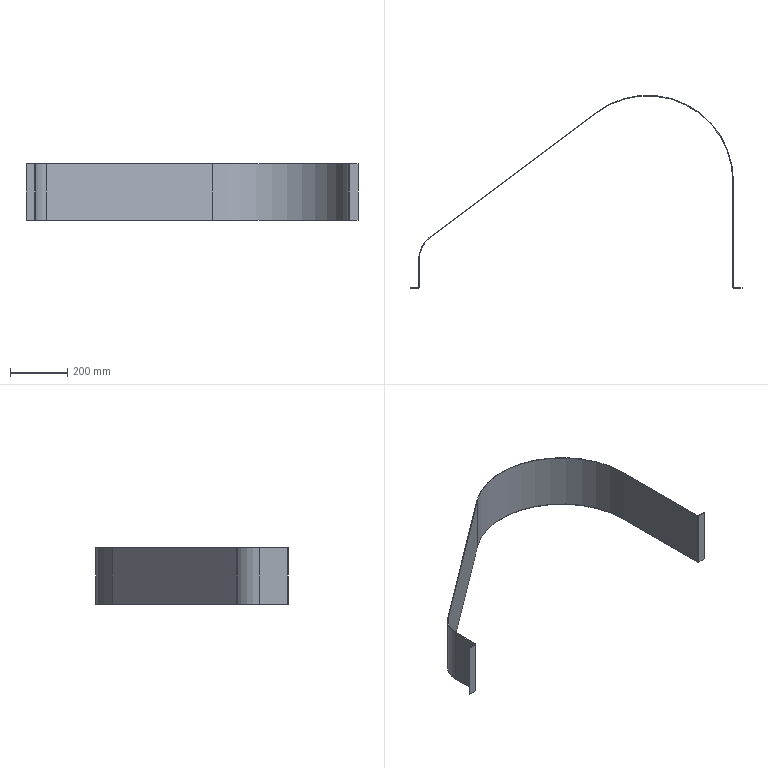Part | SolidWorks | features ICE 5, SheetMetal 3, SolidToSheetMetal 3, DeleteBody 1, Extrusion 1, FlatPattern 1, Shell 1, Split 1 | 1 solid | 38 faces | box 1160 x 675 x 198 mm | volume 796815 mm3 | plane 30 | cylinder 8 | commonest cylinder face diameters 2 x2 6 x2 196 x1 200 x1 596 x1 600 x1
STEP:
#1=CARTESIAN_POINT('',(-1098.,3.,0.));
#2=VERTEX_POINT('',#1);
#3=CARTESIAN_POINT('',(-1100.,3.,0.));
#4=VERTEX_POINT('',#3);
#5=CARTESIAN_POINT('',(-1100.,3.,0.));
#6=DIRECTION('',(-1.,0.,0.));
#7=VECTOR('',#6,1000.);
#8=LINE('',#5,#7);
#9=EDGE_CURVE('',#2,#4,#8,.T.);
#10=ORIENTED_EDGE('',*,*,#9,.F.);
#11=CARTESIAN_POINT('',(-1098.,100.,0.));
#12=VERTEX_POINT('',#11);
#13=CARTESIAN_POINT('',(-1098.,100.,0.));
#14=DIRECTION('',(0.,-1.,0.));
#15=VECTOR('',#14,1000.);
#16=LINE('',#13,#15);
#17=EDGE_CURVE('',#12,#2,#16,.T.);
#18=ORIENTED_EDGE('',*,*,#17,.F.);
#19=CARTESIAN_POINT('',(-1100.,100.,0.));
#20=VERTEX_POINT('',#19);
#21=CARTESIAN_POINT('',(-1100.,100.,0.));
#22=DIRECTION('',(-1.,0.,0.));
#23=VECTOR('',#22,1000.);
#24=LINE('',#21,#23);
#25=EDGE_CURVE('',#12,#20,#24,.T.);
#26=ORIENTED_EDGE('',*,*,#25,.T.);
#27=CARTESIAN_POINT('',(-1100.,100.,0.));
#28=DIRECTION('',(0.,-1.,0.));
#29=VECTOR('',#28,1000.);
#30=LINE('',#27,#29);
#31=EDGE_CURVE('',#20,#4,#30,.T.);
#32=ORIENTED_EDGE('',*,*,#31,.T.);
#33=EDGE_LOOP('',(#10,#18,#26,#32));
#34=FACE_OUTER_BOUND('',#33,.T.);
#35=CARTESIAN_POINT('',(-1100.,100.,0.));
#36=DIRECTION('',(0.,0.,-1.));
#37=DIRECTION('',(0.,-1.,0.));
#38=AXIS2_PLACEMENT_3D('',#35,#36,#37);
#39=PLANE('',#38);
#40=ADVANCED_FACE('',(#34),#39,.F.);
#41=ORIENTED_EDGE('',*,*,#25,.F.);
#42=CARTESIAN_POINT('',(-1058.8,178.4,0.));
#43=VERTEX_POINT('',#42);
#44=CARTESIAN_POINT('',(-1000.,100.,0.));
#45=DIRECTION('',(0.,0.,1.));
#46=DIRECTION('',(1.,0.,0.));
#47=AXIS2_PLACEMENT_3D('',#44,#45,#46);
#48=CIRCLE('',#47,98.);
#49=EDGE_CURVE('',#43,#12,#48,.T.);
#50=ORIENTED_EDGE('',*,*,#49,.F.);
#51=CARTESIAN_POINT('',(-1060.,180.,0.));
#52=VERTEX_POINT('',#51);
#53=CARTESIAN_POINT('',(-1060.,180.,0.));
#54=DIRECTION('',(-0.6,0.8,0.));
#55=VECTOR('',#54,1000.);
#56=LINE('',#53,#55);
#57=EDGE_CURVE('',#43,#52,#56,.T.);
#58=ORIENTED_EDGE('',*,*,#57,.T.);
#59=CARTESIAN_POINT('',(-1000.,100.,0.));
#60=DIRECTION('',(0.,0.,1.));
#61=DIRECTION('',(1.,0.,0.));
#62=AXIS2_PLACEMENT_3D('',#59,#60,#61);
#63=CIRCLE('',#62,100.);
#64=EDGE_CURVE('',#52,#20,#63,.T.);
#65=ORIENTED_EDGE('',*,*,#64,.T.);
#66=EDGE_LOOP('',(#41,#50,#58,#65));
#67=FACE_OUTER_BOUND('',#66,.T.);
#68=CARTESIAN_POINT('',(-1000.,100.,0.));
#69=DIRECTION('',(0.,0.,-1.));
#70=DIRECTION('',(-1.,0.,0.));
#71=AXIS2_PLACEMENT_3D('',#68,#69,#70);
#72=PLANE('',#71);
#73=ADVANCED_FACE('',(#67),#72,.F.);
#74=ORIENTED_EDGE('',*,*,#57,.F.);
#75=CARTESIAN_POINT('',(-478.8,613.4,0.));
#76=VERTEX_POINT('',#75);
#77=CARTESIAN_POINT('',(-1058.8,178.4,0.));
#78=DIRECTION('',(-0.8,-0.6,0.));
#79=VECTOR('',#78,1000.);
#80=LINE('',#77,#79);
#81=EDGE_CURVE('',#76,#43,#80,.T.);
#82=ORIENTED_EDGE('',*,*,#81,.F.);
#83=CARTESIAN_POINT('',(-480.,615.,0.));
#84=VERTEX_POINT('',#83);
#85=CARTESIAN_POINT('',(-480.,615.,0.));
#86=DIRECTION('',(-0.6,0.8,0.));
#87=VECTOR('',#86,1000.);
#88=LINE('',#85,#87);
#89=EDGE_CURVE('',#76,#84,#88,.T.);
#90=ORIENTED_EDGE('',*,*,#89,.T.);
#91=CARTESIAN_POINT('',(-1060.,180.,0.));
#92=DIRECTION('',(-0.8,-0.6,0.));
#93=VECTOR('',#92,1000.);
#94=LINE('',#91,#93);
#95=EDGE_CURVE('',#84,#52,#94,.T.);
#96=ORIENTED_EDGE('',*,*,#95,.T.);
#97=EDGE_LOOP('',(#74,#82,#90,#96));
#98=FACE_OUTER_BOUND('',#97,.T.);
#99=CARTESIAN_POINT('',(-1060.,180.,0.));
#100=DIRECTION('',(0.,0.,-1.));
#101=DIRECTION('',(-0.8,-0.6,0.));
#102=AXIS2_PLACEMENT_3D('',#99,#100,#101);
#103=PLANE('',#102);
#104=ADVANCED_FACE('',(#98),#103,.F.);
#105=ORIENTED_EDGE('',*,*,#89,.F.);
#106=CARTESIAN_POINT('',(-2.,375.,0.));
#107=VERTEX_POINT('',#106);
#108=CARTESIAN_POINT('',(-300.,375.,0.));
#109=DIRECTION('',(0.,0.,1.));
#110=DIRECTION('',(1.,0.,0.));
#111=AXIS2_PLACEMENT_3D('',#108,#109,#110);
#112=CIRCLE('',#111,298.);
#113=EDGE_CURVE('',#107,#76,#112,.T.);
#114=ORIENTED_EDGE('',*,*,#113,.F.);
#115=CARTESIAN_POINT('',(0.,375.,0.));
#116=VERTEX_POINT('',#115);
#117=CARTESIAN_POINT('',(0.,375.,0.));
#118=DIRECTION('',(1.,0.,0.));
#119=VECTOR('',#118,1000.);
#120=LINE('',#117,#119);
#121=EDGE_CURVE('',#107,#116,#120,.T.);
#122=ORIENTED_EDGE('',*,*,#121,.T.);
#123=CARTESIAN_POINT('',(-300.,375.,0.));
#124=DIRECTION('',(0.,0.,1.));
#125=DIRECTION('',(1.,0.,0.));
#126=AXIS2_PLACEMENT_3D('',#123,#124,#125);
#127=CIRCLE('',#126,300.);
#128=EDGE_CURVE('',#116,#84,#127,.T.);
#129=ORIENTED_EDGE('',*,*,#128,.T.);
#130=EDGE_LOOP('',(#105,#114,#122,#129));
#131=FACE_OUTER_BOUND('',#130,.T.);
#132=CARTESIAN_POINT('',(-300.,375.,0.));
#133=DIRECTION('',(0.,0.,-1.));
#134=DIRECTION('',(-1.,0.,0.));
#135=AXIS2_PLACEMENT_3D('',#132,#133,#134);
#136=PLANE('',#135);
#137=ADVANCED_FACE('',(#131),#136,.F.);
#138=ORIENTED_EDGE('',*,*,#121,.F.);
#139=CARTESIAN_POINT('',(-2.,3.,0.));
#140=VERTEX_POINT('',#139);
#141=CARTESIAN_POINT('',(-2.,0.,0.));
#142=DIRECTION('',(0.,1.,0.));
#143=VECTOR('',#142,1000.);
#144=LINE('',#141,#143);
#145=EDGE_CURVE('',#140,#107,#144,.T.);
#146=ORIENTED_EDGE('',*,*,#145,.F.);
#147=CARTESIAN_POINT('',(0.,3.,0.));
#148=VERTEX_POINT('',#147);
#149=CARTESIAN_POINT('',(0.,3.,0.));
#150=DIRECTION('',(1.,0.,0.));
#151=VECTOR('',#150,1000.);
#152=LINE('',#149,#151);
#153=EDGE_CURVE('',#140,#148,#152,.T.);
#154=ORIENTED_EDGE('',*,*,#153,.T.);
#155=CARTESIAN_POINT('',(0.,0.,0.));
#156=DIRECTION('',(0.,1.,0.));
#157=VECTOR('',#156,1000.);
#158=LINE('',#155,#157);
#159=EDGE_CURVE('',#148,#116,#158,.T.);
#160=ORIENTED_EDGE('',*,*,#159,.T.);
#161=EDGE_LOOP('',(#138,#146,#154,#160));
#162=FACE_OUTER_BOUND('',#161,.T.);
#163=CARTESIAN_POINT('',(0.,0.,0.));
#164=DIRECTION('',(0.,0.,-1.));
#165=DIRECTION('',(0.,1.,0.));
#166=AXIS2_PLACEMENT_3D('',#163,#164,#165);
#167=PLANE('',#166);
#168=ADVANCED_FACE('',(#162),#167,.F.);
#169=ORIENTED_EDGE('',*,*,#153,.F.);
#170=CARTESIAN_POINT('',(1.,0.,0.));
#171=VERTEX_POINT('',#170);
#172=CARTESIAN_POINT('',(1.,3.,0.));
#173=DIRECTION('',(0.,0.,1.));
#174=DIRECTION('',(1.,0.,0.));
#175=AXIS2_PLACEMENT_3D('',#172,#173,#174);
#176=CIRCLE('',#175,3.);
#177=EDGE_CURVE('',#140,#171,#176,.T.);
#178=ORIENTED_EDGE('',*,*,#177,.T.);
#179=CARTESIAN_POINT('',(1.,2.,0.));
#180=VERTEX_POINT('',#179);
#181=CARTESIAN_POINT('',(1.,2.,0.));
#182=DIRECTION('',(0.,1.,0.));
#183=VECTOR('',#182,1000.);
#184=LINE('',#181,#183);
#185=EDGE_CURVE('',#171,#180,#184,.T.);
#186=ORIENTED_EDGE('',*,*,#185,.T.);
#187=CARTESIAN_POINT('',(1.,3.,0.));
#188=DIRECTION('',(0.,0.,1.));
#189=DIRECTION('',(-1.,0.,0.));
#190=AXIS2_PLACEMENT_3D('',#187,#188,#189);
#191=CIRCLE('',#190,1.);
#192=EDGE_CURVE('',#148,#180,#191,.T.);
#193=ORIENTED_EDGE('',*,*,#192,.F.);
#194=EDGE_LOOP('',(#169,#178,#186,#193));
#195=FACE_OUTER_BOUND('',#194,.T.);
#196=CARTESIAN_POINT('',(1.,3.,0.));
#197=DIRECTION('',(0.,0.,1.));
#198=DIRECTION('',(1.,0.,0.));
#199=AXIS2_PLACEMENT_3D('',#196,#197,#198);
#200=PLANE('',#199);
#201=ADVANCED_FACE('',(#195),#200,.T.);
#202=ORIENTED_EDGE('',*,*,#185,.F.);
#203=CARTESIAN_POINT('',(30.,0.,0.));
#204=VERTEX_POINT('',#203);
#205=CARTESIAN_POINT('',(0.,0.,0.));
#206=DIRECTION('',(-1.,0.,0.));
#207=VECTOR('',#206,1000.);
#208=LINE('',#205,#207);
#209=EDGE_CURVE('',#204,#171,#208,.T.);
#210=ORIENTED_EDGE('',*,*,#209,.F.);
#211=CARTESIAN_POINT('',(30.,2.,0.));
#212=VERTEX_POINT('',#211);
#213=CARTESIAN_POINT('',(30.,2.,0.));
#214=DIRECTION('',(0.,1.,0.));
#215=VECTOR('',#214,1000.);
#216=LINE('',#213,#215);
#217=EDGE_CURVE('',#204,#212,#216,.T.);
#218=ORIENTED_EDGE('',*,*,#217,.T.);
#219=CARTESIAN_POINT('',(30.,2.,0.));
#220=DIRECTION('',(-1.,0.,0.));
#221=VECTOR('',#220,1000.);
#222=LINE('',#219,#221);
#223=EDGE_CURVE('',#212,#180,#222,.T.);
#224=ORIENTED_EDGE('',*,*,#223,.T.);
#225=EDGE_LOOP('',(#202,#210,#218,#224));
#226=FACE_OUTER_BOUND('',#225,.T.);
#227=CARTESIAN_POINT('',(30.,2.,0.));
#228=DIRECTION('',(0.,0.,-1.));
#229=DIRECTION('',(-1.,0.,0.));
#230=AXIS2_PLACEMENT_3D('',#227,#228,#229);
#231=PLANE('',#230);
#232=ADVANCED_FACE('',(#226),#231,.F.);
#233=ORIENTED_EDGE('',*,*,#217,.F.);
#234=CARTESIAN_POINT('',(30.,0.,-198.));
#235=VERTEX_POINT('',#234);
#236=CARTESIAN_POINT('',(30.,0.,0.));
#237=DIRECTION('',(0.,0.,1.));
#238=VECTOR('',#237,1000.);
#239=LINE('',#236,#238);
#240=EDGE_CURVE('',#235,#204,#239,.T.);
#241=ORIENTED_EDGE('',*,*,#240,.F.);
#242=CARTESIAN_POINT('',(30.,2.,-198.));
#243=VERTEX_POINT('',#242);
#244=CARTESIAN_POINT('',(30.,2.,-198.));
#245=DIRECTION('',(0.,1.,0.));
#246=VECTOR('',#245,1000.);
#247=LINE('',#244,#246);
#248=EDGE_CURVE('',#235,#243,#247,.T.);
#249=ORIENTED_EDGE('',*,*,#248,.T.);
#250=CARTESIAN_POINT('',(30.,2.,-230.));
#251=DIRECTION('',(0.,0.,1.));
#252=VECTOR('',#251,1000.);
#253=LINE('',#250,#252);
#254=EDGE_CURVE('',#243,#212,#253,.T.);
#255=ORIENTED_EDGE('',*,*,#254,.T.);
#256=EDGE_LOOP('',(#233,#241,#249,#255));
#257=FACE_OUTER_BOUND('',#256,.T.);
#258=CARTESIAN_POINT('',(30.,2.,-230.));
#259=DIRECTION('',(-1.,0.,0.));
#260=DIRECTION('',(0.,0.,1.));
#261=AXIS2_PLACEMENT_3D('',#258,#259,#260);
#262=PLANE('',#261);
#263=ADVANCED_FACE('',(#257),#262,.F.);
#264=ORIENTED_EDGE('',*,*,#248,.F.);
#265=CARTESIAN_POINT('',(1.,0.,-198.));
#266=VERTEX_POINT('',#265);
#267=CARTESIAN_POINT('',(0.,0.,-198.));
#268=DIRECTION('',(1.,0.,0.));
#269=VECTOR('',#268,1000.);
#270=LINE('',#267,#269);
#271=EDGE_CURVE('',#266,#235,#270,.T.);
#272=ORIENTED_EDGE('',*,*,#271,.F.);
#273=CARTESIAN_POINT('',(1.,2.,-198.));
#274=VERTEX_POINT('',#273);
#275=CARTESIAN_POINT('',(1.,2.,-198.));
#276=DIRECTION('',(0.,1.,0.));
#277=VECTOR('',#276,1000.);
#278=LINE('',#275,#277);
#279=EDGE_CURVE('',#266,#274,#278,.T.);
#280=ORIENTED_EDGE('',*,*,#279,.T.);
#281=CARTESIAN_POINT('',(0.,2.,-198.));
#282=DIRECTION('',(1.,0.,0.));
#283=VECTOR('',#282,1000.);
#284=LINE('',#281,#283);
#285=EDGE_CURVE('',#274,#243,#284,.T.);
#286=ORIENTED_EDGE('',*,*,#285,.T.);
#287=EDGE_LOOP('',(#264,#272,#280,#286));
#288=FACE_OUTER_BOUND('',#287,.T.);
#289=CARTESIAN_POINT('',(0.,2.,-198.));
#290=DIRECTION('',(0.,0.,1.));
#291=DIRECTION('',(1.,0.,0.));
#292=AXIS2_PLACEMENT_3D('',#289,#290,#291);
#293=PLANE('',#292);
#294=ADVANCED_FACE('',(#288),#293,.F.);
#295=ORIENTED_EDGE('',*,*,#279,.F.);
#296=CARTESIAN_POINT('',(-2.,3.,-198.));
#297=VERTEX_POINT('',#296);
#298=CARTESIAN_POINT('',(1.,3.,-198.));
#299=DIRECTION('',(0.,0.,-1.));
#300=DIRECTION('',(1.,0.,0.));
#301=AXIS2_PLACEMENT_3D('',#298,#299,#300);
#302=CIRCLE('',#301,3.);
#303=EDGE_CURVE('',#266,#297,#302,.T.);
#304=ORIENTED_EDGE('',*,*,#303,.T.);
#305=CARTESIAN_POINT('',(0.,3.,-198.));
#306=VERTEX_POINT('',#305);
#307=CARTESIAN_POINT('',(0.,3.,-198.));
#308=DIRECTION('',(1.,0.,0.));
#309=VECTOR('',#308,1000.);
#310=LINE('',#307,#309);
#311=EDGE_CURVE('',#297,#306,#310,.T.);
#312=ORIENTED_EDGE('',*,*,#311,.T.);
#313=CARTESIAN_POINT('',(1.,3.,-198.));
#314=DIRECTION('',(0.,0.,-1.));
#315=DIRECTION('',(1.,0.,0.));
#316=AXIS2_PLACEMENT_3D('',#313,#314,#315);
#317=CIRCLE('',#316,1.);
#318=EDGE_CURVE('',#274,#306,#317,.T.);
#319=ORIENTED_EDGE('',*,*,#318,.F.);
#320=EDGE_LOOP('',(#295,#304,#312,#319));
#321=FACE_OUTER_BOUND('',#320,.T.);
#322=CARTESIAN_POINT('',(1.,3.,-198.));
#323=DIRECTION('',(0.,0.,-1.));
#324=DIRECTION('',(-1.,0.,0.));
#325=AXIS2_PLACEMENT_3D('',#322,#323,#324);
#326=PLANE('',#325);
#327=ADVANCED_FACE('',(#321),#326,.T.);
#328=ORIENTED_EDGE('',*,*,#311,.F.);
#329=CARTESIAN_POINT('',(-2.,375.,-198.));
#330=VERTEX_POINT('',#329);
#331=CARTESIAN_POINT('',(-2.,0.,-198.));
#332=DIRECTION('',(0.,-1.,0.));
#333=VECTOR('',#332,1000.);
#334=LINE('',#331,#333);
#335=EDGE_CURVE('',#330,#297,#334,.T.);
#336=ORIENTED_EDGE('',*,*,#335,.F.);
#337=CARTESIAN_POINT('',(0.,375.,-198.));
#338=VERTEX_POINT('',#337);
#339=CARTESIAN_POINT('',(0.,375.,-198.));
#340=DIRECTION('',(1.,0.,0.));
#341=VECTOR('',#340,1000.);
#342=LINE('',#339,#341);
#343=EDGE_CURVE('',#330,#338,#342,.T.);
#344=ORIENTED_EDGE('',*,*,#343,.T.);
#345=CARTESIAN_POINT('',(0.,0.,-198.));
#346=DIRECTION('',(0.,-1.,0.));
#347=VECTOR('',#346,1000.);
#348=LINE('',#345,#347);
#349=EDGE_CURVE('',#338,#306,#348,.T.);
#350=ORIENTED_EDGE('',*,*,#349,.T.);
#351=EDGE_LOOP('',(#328,#336,#344,#350));
#352=FACE_OUTER_BOUND('',#351,.T.);
#353=CARTESIAN_POINT('',(0.,0.,-198.));
#354=DIRECTION('',(0.,0.,1.));
#355=DIRECTION('',(0.,-1.,0.));
#356=AXIS2_PLACEMENT_3D('',#353,#354,#355);
#357=PLANE('',#356);
#358=ADVANCED_FACE('',(#352),#357,.F.);
#359=ORIENTED_EDGE('',*,*,#343,.F.);
#360=CARTESIAN_POINT('',(-478.8,613.4,-198.));
#361=VERTEX_POINT('',#360);
#362=CARTESIAN_POINT('',(-300.,375.,-198.));
#363=DIRECTION('',(0.,0.,-1.));
#364=DIRECTION('',(1.,0.,0.));
#365=AXIS2_PLACEMENT_3D('',#362,#363,#364);
#366=CIRCLE('',#365,298.);
#367=EDGE_CURVE('',#361,#330,#366,.T.);
#368=ORIENTED_EDGE('',*,*,#367,.F.);
#369=CARTESIAN_POINT('',(-480.,615.,-198.));
#370=VERTEX_POINT('',#369);
#371=CARTESIAN_POINT('',(-480.,615.,-198.));
#372=DIRECTION('',(-0.6,0.8,0.));
#373=VECTOR('',#372,1000.);
#374=LINE('',#371,#373);
#375=EDGE_CURVE('',#361,#370,#374,.T.);
#376=ORIENTED_EDGE('',*,*,#375,.T.);
#377=CARTESIAN_POINT('',(-300.,375.,-198.));
#378=DIRECTION('',(0.,0.,-1.));
#379=DIRECTION('',(1.,0.,0.));
#380=AXIS2_PLACEMENT_3D('',#377,#378,#379);
#381=CIRCLE('',#380,300.);
#382=EDGE_CURVE('',#370,#338,#381,.T.);
#383=ORIENTED_EDGE('',*,*,#382,.T.);
#384=EDGE_LOOP('',(#359,#368,#376,#383));
#385=FACE_OUTER_BOUND('',#384,.T.);
#386=CARTESIAN_POINT('',(-300.,375.,-198.));
#387=DIRECTION('',(0.,0.,-1.));
#388=DIRECTION('',(-1.,0.,0.));
#389=AXIS2_PLACEMENT_3D('',#386,#387,#388);
#390=PLANE('',#389);
#391=ADVANCED_FACE('',(#385),#390,.T.);
#392=ORIENTED_EDGE('',*,*,#375,.F.);
#393=CARTESIAN_POINT('',(-1058.8,178.4,-198.));
#394=VERTEX_POINT('',#393);
#395=CARTESIAN_POINT('',(-1058.8,178.4,-198.));
#396=DIRECTION('',(0.8,0.6,0.));
#397=VECTOR('',#396,1000.);
#398=LINE('',#395,#397);
#399=EDGE_CURVE('',#394,#361,#398,.T.);
#400=ORIENTED_EDGE('',*,*,#399,.F.);
#401=CARTESIAN_POINT('',(-1060.,180.,-198.));
#402=VERTEX_POINT('',#401);
#403=CARTESIAN_POINT('',(-1060.,180.,-198.));
#404=DIRECTION('',(-0.6,0.8,0.));
#405=VECTOR('',#404,1000.);
#406=LINE('',#403,#405);
#407=EDGE_CURVE('',#394,#402,#406,.T.);
#408=ORIENTED_EDGE('',*,*,#407,.T.);
#409=CARTESIAN_POINT('',(-1060.,180.,-198.));
#410=DIRECTION('',(0.8,0.6,0.));
#411=VECTOR('',#410,1000.);
#412=LINE('',#409,#411);
#413=EDGE_CURVE('',#402,#370,#412,.T.);
#414=ORIENTED_EDGE('',*,*,#413,.T.);
#415=EDGE_LOOP('',(#392,#400,#408,#414));
#416=FACE_OUTER_BOUND('',#415,.T.);
#417=CARTESIAN_POINT('',(-1060.,180.,-198.));
#418=DIRECTION('',(0.,0.,1.));
#419=DIRECTION('',(0.8,0.6,0.));
#420=AXIS2_PLACEMENT_3D('',#417,#418,#419);
#421=PLANE('',#420);
#422=ADVANCED_FACE('',(#416),#421,.F.);
#423=ORIENTED_EDGE('',*,*,#407,.F.);
#424=CARTESIAN_POINT('',(-1098.,100.,-198.));
#425=VERTEX_POINT('',#424);
#426=CARTESIAN_POINT('',(-1000.,100.,-198.));
#427=DIRECTION('',(0.,0.,-1.));
#428=DIRECTION('',(1.,0.,0.));
#429=AXIS2_PLACEMENT_3D('',#426,#427,#428);
#430=CIRCLE('',#429,98.);
#431=EDGE_CURVE('',#425,#394,#430,.T.);
#432=ORIENTED_EDGE('',*,*,#431,.F.);
#433=CARTESIAN_POINT('',(-1100.,100.,-198.));
#434=VERTEX_POINT('',#433);
#435=CARTESIAN_POINT('',(-1100.,100.,-198.));
#436=DIRECTION('',(-1.,0.,0.));
#437=VECTOR('',#436,1000.);
#438=LINE('',#435,#437);
#439=EDGE_CURVE('',#425,#434,#438,.T.);
#440=ORIENTED_EDGE('',*,*,#439,.T.);
#441=CARTESIAN_POINT('',(-1000.,100.,-198.));
#442=DIRECTION('',(0.,0.,-1.));
#443=DIRECTION('',(1.,0.,0.));
#444=AXIS2_PLACEMENT_3D('',#441,#442,#443);
#445=CIRCLE('',#444,100.);
#446=EDGE_CURVE('',#434,#402,#445,.T.);
#447=ORIENTED_EDGE('',*,*,#446,.T.);
#448=EDGE_LOOP('',(#423,#432,#440,#447));
#449=FACE_OUTER_BOUND('',#448,.T.);
#450=CARTESIAN_POINT('',(-1000.,100.,-198.));
#451=DIRECTION('',(0.,0.,-1.));
#452=DIRECTION('',(-1.,0.,0.));
#453=AXIS2_PLACEMENT_3D('',#450,#451,#452);
#454=PLANE('',#453);
#455=ADVANCED_FACE('',(#449),#454,.T.);
#456=ORIENTED_EDGE('',*,*,#439,.F.);
#457=CARTESIAN_POINT('',(-1098.,3.,-198.));
#458=VERTEX_POINT('',#457);
#459=CARTESIAN_POINT('',(-1098.,100.,-198.));
#460=DIRECTION('',(0.,1.,0.));
#461=VECTOR('',#460,1000.);
#462=LINE('',#459,#461);
#463=EDGE_CURVE('',#458,#425,#462,.T.);
#464=ORIENTED_EDGE('',*,*,#463,.F.);
#465=CARTESIAN_POINT('',(-1100.,3.,-198.));
#466=VERTEX_POINT('',#465);
#467=CARTESIAN_POINT('',(-1100.,3.,-198.));
#468=DIRECTION('',(-1.,0.,0.));
#469=VECTOR('',#468,1000.);
#470=LINE('',#467,#469);
#471=EDGE_CURVE('',#458,#466,#470,.T.);
#472=ORIENTED_EDGE('',*,*,#471,.T.);
#473=CARTESIAN_POINT('',(-1100.,100.,-198.));
#474=DIRECTION('',(0.,1.,0.));
#475=VECTOR('',#474,1000.);
#476=LINE('',#473,#475);
#477=EDGE_CURVE('',#466,#434,#476,.T.);
#478=ORIENTED_EDGE('',*,*,#477,.T.);
#479=EDGE_LOOP('',(#456,#464,#472,#478));
#480=FACE_OUTER_BOUND('',#479,.T.);
#481=CARTESIAN_POINT('',(-1100.,100.,-198.));
#482=DIRECTION('',(0.,0.,1.));
#483=DIRECTION('',(0.,1.,0.));
#484=AXIS2_PLACEMENT_3D('',#481,#482,#483);
#485=PLANE('',#484);
#486=ADVANCED_FACE('',(#480),#485,.F.);
#487=ORIENTED_EDGE('',*,*,#471,.F.);
#488=CARTESIAN_POINT('',(-1101.,0.,-198.));
#489=VERTEX_POINT('',#488);
#490=CARTESIAN_POINT('',(-1101.,3.,-198.));
#491=DIRECTION('',(0.,0.,-1.));
#492=DIRECTION('',(-1.,0.,0.));
#493=AXIS2_PLACEMENT_3D('',#490,#491,#492);
#494=CIRCLE('',#493,3.);
#495=EDGE_CURVE('',#458,#489,#494,.T.);
#496=ORIENTED_EDGE('',*,*,#495,.T.);
#497=CARTESIAN_POINT('',(-1101.,2.,-198.));
#498=VERTEX_POINT('',#497);
#499=CARTESIAN_POINT('',(-1101.,2.,-198.));
#500=DIRECTION('',(0.,1.,0.));
#501=VECTOR('',#500,1000.);
#502=LINE('',#499,#501);
#503=EDGE_CURVE('',#489,#498,#502,.T.);
#504=ORIENTED_EDGE('',*,*,#503,.T.);
#505=CARTESIAN_POINT('',(-1101.,3.,-198.));
#506=DIRECTION('',(0.,0.,-1.));
#507=DIRECTION('',(1.,0.,0.));
#508=AXIS2_PLACEMENT_3D('',#505,#506,#507);
#509=CIRCLE('',#508,1.);
#510=EDGE_CURVE('',#466,#498,#509,.T.);
#511=ORIENTED_EDGE('',*,*,#510,.F.);
#512=EDGE_LOOP('',(#487,#496,#504,#511));
#513=FACE_OUTER_BOUND('',#512,.T.);
#514=CARTESIAN_POINT('',(-1101.,3.,-198.));
#515=DIRECTION('',(0.,0.,-1.));
#516=DIRECTION('',(-1.,0.,0.));
#517=AXIS2_PLACEMENT_3D('',#514,#515,#516);
#518=PLANE('',#517);
#519=ADVANCED_FACE('',(#513),#518,.T.);
#520=ORIENTED_EDGE('',*,*,#503,.F.);
#521=CARTESIAN_POINT('',(-1130.,0.,-198.));
#522=VERTEX_POINT('',#521);
#523=CARTESIAN_POINT('',(0.,0.,-198.));
#524=DIRECTION('',(1.,0.,0.));
#525=VECTOR('',#524,1000.);
#526=LINE('',#523,#525);
#527=EDGE_CURVE('',#522,#489,#526,.T.);
#528=ORIENTED_EDGE('',*,*,#527,.F.);
#529=CARTESIAN_POINT('',(-1130.,2.,-198.));
#530=VERTEX_POINT('',#529);
#531=CARTESIAN_POINT('',(-1130.,2.,-198.));
#532=DIRECTION('',(0.,1.,0.));
#533=VECTOR('',#532,1000.);
#534=LINE('',#531,#533);
#535=EDGE_CURVE('',#522,#530,#534,.T.);
#536=ORIENTED_EDGE('',*,*,#535,.T.);
#537=CARTESIAN_POINT('',(0.,2.,-198.));
#538=DIRECTION('',(1.,0.,0.));
#539=VECTOR('',#538,1000.);
#540=LINE('',#537,#539);
#541=EDGE_CURVE('',#530,#498,#540,.T.);
#542=ORIENTED_EDGE('',*,*,#541,.T.);
#543=EDGE_LOOP('',(#520,#528,#536,#542));
#544=FACE_OUTER_BOUND('',#543,.T.);
#545=CARTESIAN_POINT('',(0.,2.,-198.));
#546=DIRECTION('',(0.,0.,1.));
#547=DIRECTION('',(1.,0.,0.));
#548=AXIS2_PLACEMENT_3D('',#545,#546,#547);
#549=PLANE('',#548);
#550=ADVANCED_FACE('',(#544),#549,.F.);
#551=ORIENTED_EDGE('',*,*,#535,.F.);
#552=CARTESIAN_POINT('',(-1130.,0.,0.));
#553=VERTEX_POINT('',#552);
#554=CARTESIAN_POINT('',(-1130.,0.,0.));
#555=DIRECTION('',(0.,0.,-1.));
#556=VECTOR('',#555,1000.);
#557=LINE('',#554,#556);
#558=EDGE_CURVE('',#553,#522,#557,.T.);
#559=ORIENTED_EDGE('',*,*,#558,.F.);
#560=CARTESIAN_POINT('',(-1130.,2.,0.));
#561=VERTEX_POINT('',#560);
#562=CARTESIAN_POINT('',(-1130.,2.,0.));
#563=DIRECTION('',(0.,1.,0.));
#564=VECTOR('',#563,1000.);
#565=LINE('',#562,#564);
#566=EDGE_CURVE('',#553,#561,#565,.T.);
#567=ORIENTED_EDGE('',*,*,#566,.T.);
#568=CARTESIAN_POINT('',(-1130.,2.,0.));
#569=DIRECTION('',(0.,0.,-1.));
#570=VECTOR('',#569,1000.);
#571=LINE('',#568,#570);
#572=EDGE_CURVE('',#561,#530,#571,.T.);
#573=ORIENTED_EDGE('',*,*,#572,.T.);
#574=EDGE_LOOP('',(#551,#559,#567,#573));
#575=FACE_OUTER_BOUND('',#574,.T.);
#576=CARTESIAN_POINT('',(-1130.,2.,0.));
#577=DIRECTION('',(1.,0.,0.));
#578=DIRECTION('',(0.,0.,-1.));
#579=AXIS2_PLACEMENT_3D('',#576,#577,#578);
#580=PLANE('',#579);
#581=ADVANCED_FACE('',(#575),#580,.F.);
#582=ORIENTED_EDGE('',*,*,#566,.F.);
#583=CARTESIAN_POINT('',(-1101.,0.,0.));
#584=VERTEX_POINT('',#583);
#585=CARTESIAN_POINT('',(0.,0.,0.));
#586=DIRECTION('',(-1.,0.,0.));
#587=VECTOR('',#586,1000.);
#588=LINE('',#585,#587);
#589=EDGE_CURVE('',#584,#553,#588,.T.);
#590=ORIENTED_EDGE('',*,*,#589,.F.);
#591=CARTESIAN_POINT('',(-1101.,2.,0.));
#592=VERTEX_POINT('',#591);
#593=CARTESIAN_POINT('',(-1101.,2.,0.));
#594=DIRECTION('',(0.,1.,0.));
#595=VECTOR('',#594,1000.);
#596=LINE('',#593,#595);
#597=EDGE_CURVE('',#584,#592,#596,.T.);
#598=ORIENTED_EDGE('',*,*,#597,.T.);
#599=CARTESIAN_POINT('',(-1100.,2.,0.));
#600=DIRECTION('',(-1.,0.,0.));
#601=VECTOR('',#600,1000.);
#602=LINE('',#599,#601);
#603=EDGE_CURVE('',#592,#561,#602,.T.);
#604=ORIENTED_EDGE('',*,*,#603,.T.);
#605=EDGE_LOOP('',(#582,#590,#598,#604));
#606=FACE_OUTER_BOUND('',#605,.T.);
#607=CARTESIAN_POINT('',(-1100.,2.,0.));
#608=DIRECTION('',(0.,0.,-1.));
#609=DIRECTION('',(-1.,0.,0.));
#610=AXIS2_PLACEMENT_3D('',#607,#608,#609);
#611=PLANE('',#610);
#612=ADVANCED_FACE('',(#606),#611,.F.);
#613=CARTESIAN_POINT('',(-1101.,3.,0.));
#614=DIRECTION('',(0.,0.,1.));
#615=DIRECTION('',(-1.,0.,0.));
#616=AXIS2_PLACEMENT_3D('',#613,#614,#615);
#617=CIRCLE('',#616,3.);
#618=EDGE_CURVE('',#584,#2,#617,.T.);
#619=ORIENTED_EDGE('',*,*,#618,.T.);
#620=ORIENTED_EDGE('',*,*,#9,.T.);
#621=CARTESIAN_POINT('',(-1101.,3.,0.));
#622=DIRECTION('',(0.,0.,1.));
#623=DIRECTION('',(-1.,0.,0.));
#624=AXIS2_PLACEMENT_3D('',#621,#622,#623);
#625=CIRCLE('',#624,1.);
#626=EDGE_CURVE('',#592,#4,#625,.T.);
#627=ORIENTED_EDGE('',*,*,#626,.F.);
#628=ORIENTED_EDGE('',*,*,#597,.F.);
#629=EDGE_LOOP('',(#619,#620,#627,#628));
#630=FACE_OUTER_BOUND('',#629,.T.);
#631=CARTESIAN_POINT('',(-1101.,3.,0.));
#632=DIRECTION('',(0.,0.,1.));
#633=DIRECTION('',(1.,0.,0.));
#634=AXIS2_PLACEMENT_3D('',#631,#632,#633);
#635=PLANE('',#634);
#636=ADVANCED_FACE('',(#630),#635,.T.);
#637=ORIENTED_EDGE('',*,*,#603,.F.);
#638=CARTESIAN_POINT('',(-1101.,2.,-198.));
#639=DIRECTION('',(0.,0.,-1.));
#640=VECTOR('',#639,1000.);
#641=LINE('',#638,#640);
#642=EDGE_CURVE('',#592,#498,#641,.T.);
#643=ORIENTED_EDGE('',*,*,#642,.T.);
#644=ORIENTED_EDGE('',*,*,#541,.F.);
#645=ORIENTED_EDGE('',*,*,#572,.F.);
#646=EDGE_LOOP('',(#637,#643,#644,#645));
#647=FACE_OUTER_BOUND('',#646,.T.);
#648=CARTESIAN_POINT('',(0.,2.,0.));
#649=DIRECTION('',(0.,1.,0.));
#650=DIRECTION('',(0.,0.,1.));
#651=AXIS2_PLACEMENT_3D('',#648,#649,#650);
#652=PLANE('',#651);
#653=ADVANCED_FACE('',(#647),#652,.T.);
#654=ORIENTED_EDGE('',*,*,#446,.F.);
#655=CARTESIAN_POINT('',(-1100.,100.,-200.));
#656=DIRECTION('',(0.,0.,1.));
#657=VECTOR('',#656,1000.);
#658=LINE('',#655,#657);
#659=EDGE_CURVE('',#434,#20,#658,.T.);
#660=ORIENTED_EDGE('',*,*,#659,.T.);
#661=ORIENTED_EDGE('',*,*,#64,.F.);
#662=CARTESIAN_POINT('',(-1060.,180.,-200.));
#663=DIRECTION('',(0.,0.,1.));
#664=VECTOR('',#663,1000.);
#665=LINE('',#662,#664);
#666=EDGE_CURVE('',#402,#52,#665,.T.);
#667=ORIENTED_EDGE('',*,*,#666,.F.);
#668=EDGE_LOOP('',(#654,#660,#661,#667));
#669=FACE_OUTER_BOUND('',#668,.T.);
#670=CARTESIAN_POINT('',(-1000.,100.,-200.));
#671=DIRECTION('',(0.,0.,1.));
#672=DIRECTION('',(1.,0.,0.));
#673=AXIS2_PLACEMENT_3D('',#670,#671,#672);
#674=CYLINDRICAL_SURFACE('',#673,100.);
#675=ADVANCED_FACE('',(#669),#674,.T.);
#676=ORIENTED_EDGE('',*,*,#477,.F.);
#677=CARTESIAN_POINT('',(-1100.,3.,0.));
#678=DIRECTION('',(0.,0.,1.));
#679=VECTOR('',#678,1000.);
#680=LINE('',#677,#679);
#681=EDGE_CURVE('',#466,#4,#680,.T.);
#682=ORIENTED_EDGE('',*,*,#681,.T.);
#683=ORIENTED_EDGE('',*,*,#31,.F.);
#684=ORIENTED_EDGE('',*,*,#659,.F.);
#685=EDGE_LOOP('',(#676,#682,#683,#684));
#686=FACE_OUTER_BOUND('',#685,.T.);
#687=CARTESIAN_POINT('',(-1100.,100.,-200.));
#688=DIRECTION('',(-1.,0.,0.));
#689=DIRECTION('',(0.,0.,1.));
#690=AXIS2_PLACEMENT_3D('',#687,#688,#689);
#691=PLANE('',#690);
#692=ADVANCED_FACE('',(#686),#691,.T.);
#693=ORIENTED_EDGE('',*,*,#382,.F.);
#694=CARTESIAN_POINT('',(-480.,615.,-200.));
#695=DIRECTION('',(0.,0.,1.));
#696=VECTOR('',#695,1000.);
#697=LINE('',#694,#696);
#698=EDGE_CURVE('',#370,#84,#697,.T.);
#699=ORIENTED_EDGE('',*,*,#698,.T.);
#700=ORIENTED_EDGE('',*,*,#128,.F.);
#701=CARTESIAN_POINT('',(0.,375.,-200.));
#702=DIRECTION('',(0.,0.,1.));
#703=VECTOR('',#702,1000.);
#704=LINE('',#701,#703);
#705=EDGE_CURVE('',#338,#116,#704,.T.);
#706=ORIENTED_EDGE('',*,*,#705,.F.);
#707=EDGE_LOOP('',(#693,#699,#700,#706));
#708=FACE_OUTER_BOUND('',#707,.T.);
#709=CARTESIAN_POINT('',(-300.,375.,-200.));
#710=DIRECTION('',(0.,0.,1.));
#711=DIRECTION('',(1.,0.,0.));
#712=AXIS2_PLACEMENT_3D('',#709,#710,#711);
#713=CYLINDRICAL_SURFACE('',#712,300.);
#714=ADVANCED_FACE('',(#708),#713,.T.);
#715=ORIENTED_EDGE('',*,*,#413,.F.);
#716=ORIENTED_EDGE('',*,*,#666,.T.);
#717=ORIENTED_EDGE('',*,*,#95,.F.);
#718=ORIENTED_EDGE('',*,*,#698,.F.);
#719=EDGE_LOOP('',(#715,#716,#717,#718));
#720=FACE_OUTER_BOUND('',#719,.T.);
#721=CARTESIAN_POINT('',(-1060.,180.,-200.));
#722=DIRECTION('',(-0.6,0.8,0.));
#723=DIRECTION('',(-0.8,-0.6,0.));
#724=AXIS2_PLACEMENT_3D('',#721,#722,#723);
#725=PLANE('',#724);
#726=ADVANCED_FACE('',(#720),#725,.T.);
#727=ORIENTED_EDGE('',*,*,#285,.F.);
#728=CARTESIAN_POINT('',(1.,2.,0.));
#729=DIRECTION('',(0.,0.,1.));
#730=VECTOR('',#729,1000.);
#731=LINE('',#728,#730);
#732=EDGE_CURVE('',#274,#180,#731,.T.);
#733=ORIENTED_EDGE('',*,*,#732,.T.);
#734=ORIENTED_EDGE('',*,*,#223,.F.);
#735=ORIENTED_EDGE('',*,*,#254,.F.);
#736=EDGE_LOOP('',(#727,#733,#734,#735));
#737=FACE_OUTER_BOUND('',#736,.T.);
#738=CARTESIAN_POINT('',(0.,2.,0.));
#739=DIRECTION('',(0.,1.,0.));
#740=DIRECTION('',(0.,0.,1.));
#741=AXIS2_PLACEMENT_3D('',#738,#739,#740);
#742=PLANE('',#741);
#743=ADVANCED_FACE('',(#737),#742,.T.);
#744=ORIENTED_EDGE('',*,*,#159,.F.);
#745=CARTESIAN_POINT('',(0.,3.,-198.));
#746=DIRECTION('',(0.,0.,-1.));
#747=VECTOR('',#746,1000.);
#748=LINE('',#745,#747);
#749=EDGE_CURVE('',#148,#306,#748,.T.);
#750=ORIENTED_EDGE('',*,*,#749,.T.);
#751=ORIENTED_EDGE('',*,*,#349,.F.);
#752=ORIENTED_EDGE('',*,*,#705,.T.);
#753=EDGE_LOOP('',(#744,#750,#751,#752));
#754=FACE_OUTER_BOUND('',#753,.T.);
#755=CARTESIAN_POINT('',(0.,0.,-200.));
#756=DIRECTION('',(1.,0.,0.));
#757=DIRECTION('',(0.,0.,-1.));
#758=AXIS2_PLACEMENT_3D('',#755,#756,#757);
#759=PLANE('',#758);
#760=ADVANCED_FACE('',(#754),#759,.T.);
#761=ORIENTED_EDGE('',*,*,#510,.T.);
#762=ORIENTED_EDGE('',*,*,#642,.F.);
#763=ORIENTED_EDGE('',*,*,#626,.T.);
#764=ORIENTED_EDGE('',*,*,#681,.F.);
#765=EDGE_LOOP('',(#761,#762,#763,#764));
#766=FACE_OUTER_BOUND('',#765,.T.);
#767=CARTESIAN_POINT('',(-1101.,3.,-200.));
#768=DIRECTION('',(0.,0.,-1.));
#769=DIRECTION('',(-1.,0.,0.));
#770=AXIS2_PLACEMENT_3D('',#767,#768,#769);
#771=CYLINDRICAL_SURFACE('',#770,1.);
#772=ADVANCED_FACE('',(#766),#771,.F.);
#773=ORIENTED_EDGE('',*,*,#192,.T.);
#774=ORIENTED_EDGE('',*,*,#732,.F.);
#775=ORIENTED_EDGE('',*,*,#318,.T.);
#776=ORIENTED_EDGE('',*,*,#749,.F.);
#777=EDGE_LOOP('',(#773,#774,#775,#776));
#778=FACE_OUTER_BOUND('',#777,.T.);
#779=CARTESIAN_POINT('',(1.,3.,-200.));
#780=DIRECTION('',(0.,0.,1.));
#781=DIRECTION('',(1.,0.,0.));
#782=AXIS2_PLACEMENT_3D('',#779,#780,#781);
#783=CYLINDRICAL_SURFACE('',#782,1.);
#784=ADVANCED_FACE('',(#778),#783,.F.);
#785=ORIENTED_EDGE('',*,*,#589,.T.);
#786=ORIENTED_EDGE('',*,*,#558,.T.);
#787=ORIENTED_EDGE('',*,*,#527,.T.);
#788=CARTESIAN_POINT('',(-1101.,0.,0.));
#789=DIRECTION('',(0.,0.,-1.));
#790=VECTOR('',#789,1000.);
#791=LINE('',#788,#790);
#792=EDGE_CURVE('',#584,#489,#791,.T.);
#793=ORIENTED_EDGE('',*,*,#792,.F.);
#794=EDGE_LOOP('',(#785,#786,#787,#793));
#795=FACE_OUTER_BOUND('',#794,.T.);
#796=CARTESIAN_POINT('',(0.,0.,0.));
#797=DIRECTION('',(0.,1.,0.));
#798=DIRECTION('',(0.,0.,1.));
#799=AXIS2_PLACEMENT_3D('',#796,#797,#798);
#800=PLANE('',#799);
#801=ADVANCED_FACE('',(#795),#800,.F.);
#802=ORIENTED_EDGE('',*,*,#431,.T.);
#803=CARTESIAN_POINT('',(-1058.8,178.4,-200.));
#804=DIRECTION('',(0.,0.,1.));
#805=VECTOR('',#804,1000.);
#806=LINE('',#803,#805);
#807=EDGE_CURVE('',#394,#43,#806,.T.);
#808=ORIENTED_EDGE('',*,*,#807,.T.);
#809=ORIENTED_EDGE('',*,*,#49,.T.);
#810=CARTESIAN_POINT('',(-1098.,100.,-200.));
#811=DIRECTION('',(0.,0.,1.));
#812=VECTOR('',#811,1000.);
#813=LINE('',#810,#812);
#814=EDGE_CURVE('',#425,#12,#813,.T.);
#815=ORIENTED_EDGE('',*,*,#814,.F.);
#816=EDGE_LOOP('',(#802,#808,#809,#815));
#817=FACE_OUTER_BOUND('',#816,.T.);
#818=CARTESIAN_POINT('',(-1000.,100.,-200.));
#819=DIRECTION('',(0.,0.,1.));
#820=DIRECTION('',(1.,0.,0.));
#821=AXIS2_PLACEMENT_3D('',#818,#819,#820);
#822=CYLINDRICAL_SURFACE('',#821,98.);
#823=ADVANCED_FACE('',(#817),#822,.F.);
#824=ORIENTED_EDGE('',*,*,#463,.T.);
#825=ORIENTED_EDGE('',*,*,#814,.T.);
#826=ORIENTED_EDGE('',*,*,#17,.T.);
#827=CARTESIAN_POINT('',(-1098.,3.,-200.));
#828=DIRECTION('',(0.,0.,1.));
#829=VECTOR('',#828,1000.);
#830=LINE('',#827,#829);
#831=EDGE_CURVE('',#458,#2,#830,.T.);
#832=ORIENTED_EDGE('',*,*,#831,.F.);
#833=EDGE_LOOP('',(#824,#825,#826,#832));
#834=FACE_OUTER_BOUND('',#833,.T.);
#835=CARTESIAN_POINT('',(-1098.,100.,-200.));
#836=DIRECTION('',(-1.,0.,0.));
#837=DIRECTION('',(0.,0.,1.));
#838=AXIS2_PLACEMENT_3D('',#835,#836,#837);
#839=PLANE('',#838);
#840=ADVANCED_FACE('',(#834),#839,.F.);
#841=ORIENTED_EDGE('',*,*,#367,.T.);
#842=CARTESIAN_POINT('',(-2.,375.,-200.));
#843=DIRECTION('',(0.,0.,1.));
#844=VECTOR('',#843,1000.);
#845=LINE('',#842,#844);
#846=EDGE_CURVE('',#330,#107,#845,.T.);
#847=ORIENTED_EDGE('',*,*,#846,.T.);
#848=ORIENTED_EDGE('',*,*,#113,.T.);
#849=CARTESIAN_POINT('',(-478.8,613.4,-200.));
#850=DIRECTION('',(0.,0.,1.));
#851=VECTOR('',#850,1000.);
#852=LINE('',#849,#851);
#853=EDGE_CURVE('',#361,#76,#852,.T.);
#854=ORIENTED_EDGE('',*,*,#853,.F.);
#855=EDGE_LOOP('',(#841,#847,#848,#854));
#856=FACE_OUTER_BOUND('',#855,.T.);
#857=CARTESIAN_POINT('',(-300.,375.,-200.));
#858=DIRECTION('',(0.,0.,1.));
#859=DIRECTION('',(1.,0.,0.));
#860=AXIS2_PLACEMENT_3D('',#857,#858,#859);
#861=CYLINDRICAL_SURFACE('',#860,298.);
#862=ADVANCED_FACE('',(#856),#861,.F.);
#863=ORIENTED_EDGE('',*,*,#399,.T.);
#864=ORIENTED_EDGE('',*,*,#853,.T.);
#865=ORIENTED_EDGE('',*,*,#81,.T.);
#866=ORIENTED_EDGE('',*,*,#807,.F.);
#867=EDGE_LOOP('',(#863,#864,#865,#866));
#868=FACE_OUTER_BOUND('',#867,.T.);
#869=CARTESIAN_POINT('',(-1058.8,178.4,-200.));
#870=DIRECTION('',(-0.6,0.8,0.));
#871=DIRECTION('',(-0.8,-0.6,0.));
#872=AXIS2_PLACEMENT_3D('',#869,#870,#871);
#873=PLANE('',#872);
#874=ADVANCED_FACE('',(#868),#873,.F.);
#875=ORIENTED_EDGE('',*,*,#271,.T.);
#876=ORIENTED_EDGE('',*,*,#240,.T.);
#877=ORIENTED_EDGE('',*,*,#209,.T.);
#878=CARTESIAN_POINT('',(1.,0.,0.));
#879=DIRECTION('',(0.,0.,1.));
#880=VECTOR('',#879,1000.);
#881=LINE('',#878,#880);
#882=EDGE_CURVE('',#266,#171,#881,.T.);
#883=ORIENTED_EDGE('',*,*,#882,.F.);
#884=EDGE_LOOP('',(#875,#876,#877,#883));
#885=FACE_OUTER_BOUND('',#884,.T.);
#886=CARTESIAN_POINT('',(0.,0.,0.));
#887=DIRECTION('',(0.,1.,0.));
#888=DIRECTION('',(0.,0.,1.));
#889=AXIS2_PLACEMENT_3D('',#886,#887,#888);
#890=PLANE('',#889);
#891=ADVANCED_FACE('',(#885),#890,.F.);
#892=ORIENTED_EDGE('',*,*,#145,.T.);
#893=ORIENTED_EDGE('',*,*,#846,.F.);
#894=ORIENTED_EDGE('',*,*,#335,.T.);
#895=CARTESIAN_POINT('',(-2.,3.,-200.));
#896=DIRECTION('',(0.,0.,-1.));
#897=VECTOR('',#896,1000.);
#898=LINE('',#895,#897);
#899=EDGE_CURVE('',#140,#297,#898,.T.);
#900=ORIENTED_EDGE('',*,*,#899,.F.);
#901=EDGE_LOOP('',(#892,#893,#894,#900));
#902=FACE_OUTER_BOUND('',#901,.T.);
#903=CARTESIAN_POINT('',(-2.,0.,-200.));
#904=DIRECTION('',(1.,0.,0.));
#905=DIRECTION('',(0.,0.,-1.));
#906=AXIS2_PLACEMENT_3D('',#903,#904,#905);
#907=PLANE('',#906);
#908=ADVANCED_FACE('',(#902),#907,.F.);
#909=ORIENTED_EDGE('',*,*,#495,.F.);
#910=ORIENTED_EDGE('',*,*,#831,.T.);
#911=ORIENTED_EDGE('',*,*,#618,.F.);
#912=ORIENTED_EDGE('',*,*,#792,.T.);
#913=EDGE_LOOP('',(#909,#910,#911,#912));
#914=FACE_OUTER_BOUND('',#913,.T.);
#915=CARTESIAN_POINT('',(-1101.,3.,-200.));
#916=DIRECTION('',(0.,0.,-1.));
#917=DIRECTION('',(-1.,0.,0.));
#918=AXIS2_PLACEMENT_3D('',#915,#916,#917);
#919=CYLINDRICAL_SURFACE('',#918,3.);
#920=ADVANCED_FACE('',(#914),#919,.T.);
#921=ORIENTED_EDGE('',*,*,#177,.F.);
#922=ORIENTED_EDGE('',*,*,#899,.T.);
#923=ORIENTED_EDGE('',*,*,#303,.F.);
#924=ORIENTED_EDGE('',*,*,#882,.T.);
#925=EDGE_LOOP('',(#921,#922,#923,#924));
#926=FACE_OUTER_BOUND('',#925,.T.);
#927=CARTESIAN_POINT('',(1.,3.,-200.));
#928=DIRECTION('',(0.,0.,1.));
#929=DIRECTION('',(1.,0.,0.));
#930=AXIS2_PLACEMENT_3D('',#927,#928,#929);
#931=CYLINDRICAL_SURFACE('',#930,3.);
#932=ADVANCED_FACE('',(#926),#931,.T.);
#933=CLOSED_SHELL('',(#40,#73,#104,#137,#168,#201,#232,#263,#294,#327,#358,#391,#422,#455,#486,#519,#550,#581,#612,#636,#653,#675,#692,#714,#726,#743,#760,#772,#784,#801,#823,#840,#862,#874,#891,#908,#920,#932));
#934=MANIFOLD_SOLID_BREP('',#933);
#935=CARTESIAN_POINT('',(0.,0.,0.));
#936=DIRECTION('',(0.,0.,1.));
#937=DIRECTION('',(1.,0.,0.));
#938=AXIS2_PLACEMENT_3D('',#935,#936,#937);
#939=(LENGTH_UNIT()NAMED_UNIT(*)SI_UNIT(.MILLI.,.METRE.));
#940=UNCERTAINTY_MEASURE_WITH_UNIT(LENGTH_MEASURE(0.00001),#939,'','');
#941=(NAMED_UNIT(*)PLANE_ANGLE_UNIT()SI_UNIT($,.RADIAN.));
#942=(NAMED_UNIT(*)SI_UNIT($,.STERADIAN.)SOLID_ANGLE_UNIT());
#943=(GEOMETRIC_REPRESENTATION_CONTEXT(3)GLOBAL_UNCERTAINTY_ASSIGNED_CONTEXT((#940))GLOBAL_UNIT_ASSIGNED_CONTEXT((#939,#941,#942))REPRESENTATION_CONTEXT('',''));
#944=ADVANCED_BREP_SHAPE_REPRESENTATION('',(#934,#938),#943);